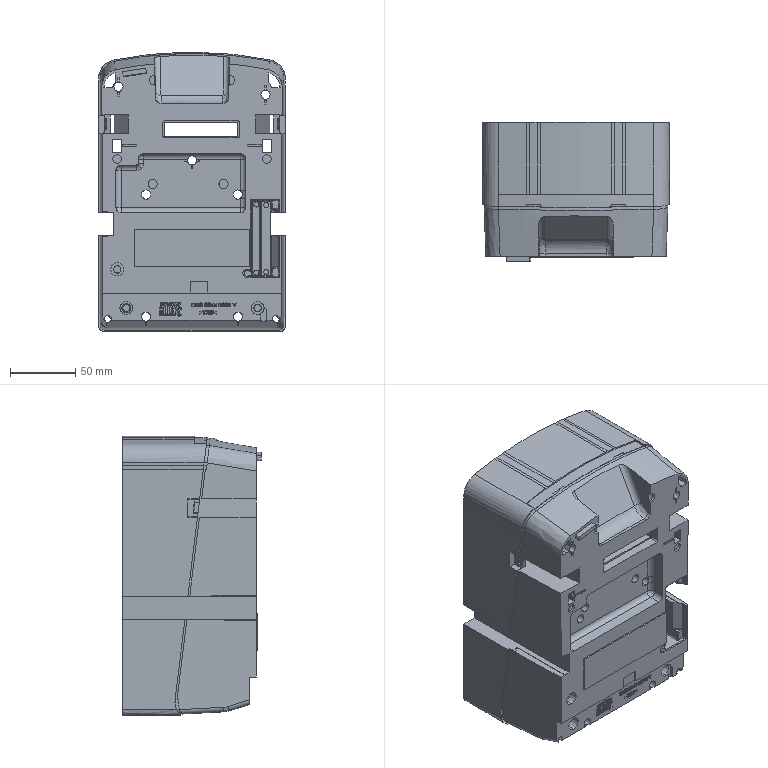Part | STEP file | 1 solid | 1708 faces | box 143.116 x 106.38 x 213.742 mm | volume 2647333 mm3 | plane 1312 | spline 201 | cylinder 130 | cone 42 | sphere 23 | commonest cylinder face diameters 1.005 x28 1.608 x27 7.035 x18 7 x14 2.01 x13 8.04 x12